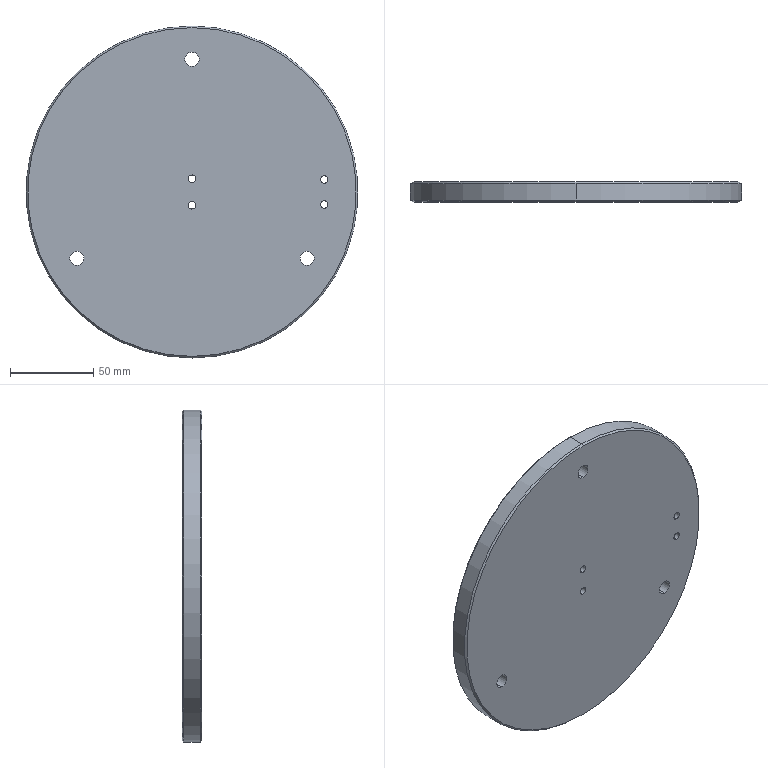Part | SolidWorks | features 3DProfileFeature 2, HoleWzd 2, Chamfer 1, Extrusion 1 | 1 solid | 34 faces | box 200 x 12 x 200 mm | volume 372597 mm3 | cylinder 24 | plane 6 | cone 4 | commonest cylinder face diameters 4.5 x8 8 x8 8.5 x6 200 x2
STEP:
#1=CARTESIAN_POINT('',(0.,-12.,-99.));
#2=VERTEX_POINT('',#1);
#3=CARTESIAN_POINT('',(0.,-12.,99.));
#4=VERTEX_POINT('',#3);
#5=CARTESIAN_POINT('',(0.,-12.,0.));
#6=DIRECTION('',(0.,-1.,0.));
#7=DIRECTION('',(0.,0.,1.));
#8=AXIS2_PLACEMENT_3D('',#5,#6,#7);
#9=CIRCLE('',#8,99.);
#10=EDGE_CURVE('',#2,#4,#9,.T.);
#11=ORIENTED_EDGE('',*,*,#10,.F.);
#12=CARTESIAN_POINT('',(0.,-11.,-100.));
#13=VERTEX_POINT('',#12);
#14=CARTESIAN_POINT('',(0.,-11.,-100.));
#15=DIRECTION('',(0.,0.7071,-0.7071));
#16=VECTOR('',#15,1000.);
#17=LINE('',#14,#16);
#18=EDGE_CURVE('',#2,#13,#17,.T.);
#19=ORIENTED_EDGE('',*,*,#18,.T.);
#20=CARTESIAN_POINT('',(0.,-11.,100.));
#21=VERTEX_POINT('',#20);
#22=CARTESIAN_POINT('',(0.,-11.,0.));
#23=DIRECTION('',(0.,1.,0.));
#24=DIRECTION('',(0.,0.,1.));
#25=AXIS2_PLACEMENT_3D('',#22,#23,#24);
#26=CIRCLE('',#25,100.);
#27=EDGE_CURVE('',#21,#13,#26,.T.);
#28=ORIENTED_EDGE('',*,*,#27,.F.);
#29=CARTESIAN_POINT('',(0.,-11.,100.));
#30=DIRECTION('',(0.,0.7071,0.7071));
#31=VECTOR('',#30,1000.);
#32=LINE('',#29,#31);
#33=EDGE_CURVE('',#4,#21,#32,.T.);
#34=ORIENTED_EDGE('',*,*,#33,.F.);
#35=EDGE_LOOP('',(#11,#19,#28,#34));
#36=FACE_OUTER_BOUND('',#35,.T.);
#37=CARTESIAN_POINT('',(0.,-11.,0.));
#38=DIRECTION('',(0.,1.,0.));
#39=DIRECTION('',(0.,0.,1.));
#40=AXIS2_PLACEMENT_3D('',#37,#38,#39);
#41=CONICAL_SURFACE('',#40,100.,0.7854);
#42=ADVANCED_FACE('',(#36),#41,.T.);
#43=CARTESIAN_POINT('',(0.,0.,99.));
#44=VERTEX_POINT('',#43);
#45=CARTESIAN_POINT('',(0.,0.,-99.));
#46=VERTEX_POINT('',#45);
#47=CARTESIAN_POINT('',(0.,0.,0.));
#48=DIRECTION('',(0.,1.,0.));
#49=DIRECTION('',(0.,0.,1.));
#50=AXIS2_PLACEMENT_3D('',#47,#48,#49);
#51=CIRCLE('',#50,99.);
#52=EDGE_CURVE('',#44,#46,#51,.T.);
#53=ORIENTED_EDGE('',*,*,#52,.F.);
#54=CARTESIAN_POINT('',(0.,-1.,100.));
#55=VERTEX_POINT('',#54);
#56=CARTESIAN_POINT('',(0.,0.,99.));
#57=DIRECTION('',(0.,-0.7071,0.7071));
#58=VECTOR('',#57,1000.);
#59=LINE('',#56,#58);
#60=EDGE_CURVE('',#44,#55,#59,.T.);
#61=ORIENTED_EDGE('',*,*,#60,.T.);
#62=CARTESIAN_POINT('',(0.,-1.,-100.));
#63=VERTEX_POINT('',#62);
#64=CARTESIAN_POINT('',(0.,-1.,0.));
#65=DIRECTION('',(0.,-1.,0.));
#66=DIRECTION('',(0.,0.,1.));
#67=AXIS2_PLACEMENT_3D('',#64,#65,#66);
#68=CIRCLE('',#67,100.);
#69=EDGE_CURVE('',#63,#55,#68,.T.);
#70=ORIENTED_EDGE('',*,*,#69,.F.);
#71=CARTESIAN_POINT('',(0.,0.,-99.));
#72=DIRECTION('',(0.,-0.7071,-0.7071));
#73=VECTOR('',#72,1000.);
#74=LINE('',#71,#73);
#75=EDGE_CURVE('',#46,#63,#74,.T.);
#76=ORIENTED_EDGE('',*,*,#75,.F.);
#77=EDGE_LOOP('',(#53,#61,#70,#76));
#78=FACE_OUTER_BOUND('',#77,.T.);
#79=CARTESIAN_POINT('',(0.,0.,0.));
#80=DIRECTION('',(0.,-1.,0.));
#81=DIRECTION('',(0.,0.,-1.));
#82=AXIS2_PLACEMENT_3D('',#79,#80,#81);
#83=CONICAL_SURFACE('',#82,99.,0.7854);
#84=ADVANCED_FACE('',(#78),#83,.T.);
#85=CARTESIAN_POINT('',(79.648,-7.,-11.5));
#86=VERTEX_POINT('',#85);
#87=CARTESIAN_POINT('',(79.648,-7.,-3.5));
#88=VERTEX_POINT('',#87);
#89=CARTESIAN_POINT('',(79.648,-7.,-7.5));
#90=DIRECTION('',(0.,1.,0.));
#91=DIRECTION('',(0.,0.,1.));
#92=AXIS2_PLACEMENT_3D('',#89,#90,#91);
#93=CIRCLE('',#92,4.);
#94=EDGE_CURVE('',#86,#88,#93,.T.);
#95=ORIENTED_EDGE('',*,*,#94,.F.);
#96=CARTESIAN_POINT('',(79.648,0.,-11.5));
#97=VERTEX_POINT('',#96);
#98=CARTESIAN_POINT('',(79.648,0.,-11.5));
#99=DIRECTION('',(0.,1.,0.));
#100=VECTOR('',#99,1000.);
#101=LINE('',#98,#100);
#102=EDGE_CURVE('',#86,#97,#101,.T.);
#103=ORIENTED_EDGE('',*,*,#102,.T.);
#104=CARTESIAN_POINT('',(79.648,0.,-3.5));
#105=VERTEX_POINT('',#104);
#106=CARTESIAN_POINT('',(79.648,0.,-7.5));
#107=DIRECTION('',(0.,1.,0.));
#108=DIRECTION('',(0.,0.,1.));
#109=AXIS2_PLACEMENT_3D('',#106,#107,#108);
#110=CIRCLE('',#109,4.);
#111=EDGE_CURVE('',#97,#105,#110,.T.);
#112=ORIENTED_EDGE('',*,*,#111,.T.);
#113=CARTESIAN_POINT('',(79.648,0.,-3.5));
#114=DIRECTION('',(0.,1.,0.));
#115=VECTOR('',#114,1000.);
#116=LINE('',#113,#115);
#117=EDGE_CURVE('',#88,#105,#116,.T.);
#118=ORIENTED_EDGE('',*,*,#117,.F.);
#119=EDGE_LOOP('',(#95,#103,#112,#118));
#120=FACE_OUTER_BOUND('',#119,.T.);
#121=CARTESIAN_POINT('',(79.648,0.,-7.5));
#122=DIRECTION('',(0.,1.,0.));
#123=DIRECTION('',(0.,0.,1.));
#124=AXIS2_PLACEMENT_3D('',#121,#122,#123);
#125=CYLINDRICAL_SURFACE('',#124,4.);
#126=ADVANCED_FACE('',(#120),#125,.F.);
#127=CARTESIAN_POINT('',(79.648,-12.,-9.75));
#128=VERTEX_POINT('',#127);
#129=CARTESIAN_POINT('',(79.648,-12.,-5.25));
#130=VERTEX_POINT('',#129);
#131=CARTESIAN_POINT('',(79.648,-12.,-7.5));
#132=DIRECTION('',(0.,1.,0.));
#133=DIRECTION('',(0.,0.,1.));
#134=AXIS2_PLACEMENT_3D('',#131,#132,#133);
#135=CIRCLE('',#134,2.25);
#136=EDGE_CURVE('',#128,#130,#135,.T.);
#137=ORIENTED_EDGE('',*,*,#136,.F.);
#138=CARTESIAN_POINT('',(79.648,-7.,-9.75));
#139=VERTEX_POINT('',#138);
#140=CARTESIAN_POINT('',(79.648,0.,-9.75));
#141=DIRECTION('',(0.,1.,0.));
#142=VECTOR('',#141,1000.);
#143=LINE('',#140,#142);
#144=EDGE_CURVE('',#128,#139,#143,.T.);
#145=ORIENTED_EDGE('',*,*,#144,.T.);
#146=CARTESIAN_POINT('',(79.648,-7.,-5.25));
#147=VERTEX_POINT('',#146);
#148=CARTESIAN_POINT('',(79.648,-7.,-7.5));
#149=DIRECTION('',(0.,1.,0.));
#150=DIRECTION('',(0.,0.,1.));
#151=AXIS2_PLACEMENT_3D('',#148,#149,#150);
#152=CIRCLE('',#151,2.25);
#153=EDGE_CURVE('',#139,#147,#152,.T.);
#154=ORIENTED_EDGE('',*,*,#153,.T.);
#155=CARTESIAN_POINT('',(79.648,0.,-5.25));
#156=DIRECTION('',(0.,1.,0.));
#157=VECTOR('',#156,1000.);
#158=LINE('',#155,#157);
#159=EDGE_CURVE('',#130,#147,#158,.T.);
#160=ORIENTED_EDGE('',*,*,#159,.F.);
#161=EDGE_LOOP('',(#137,#145,#154,#160));
#162=FACE_OUTER_BOUND('',#161,.T.);
#163=CARTESIAN_POINT('',(79.648,0.,-7.5));
#164=DIRECTION('',(0.,1.,0.));
#165=DIRECTION('',(0.,0.,1.));
#166=AXIS2_PLACEMENT_3D('',#163,#164,#165);
#167=CYLINDRICAL_SURFACE('',#166,2.25);
#168=ADVANCED_FACE('',(#162),#167,.F.);
#169=CARTESIAN_POINT('',(79.648,-7.,3.5));
#170=VERTEX_POINT('',#169);
#171=CARTESIAN_POINT('',(79.648,-7.,11.5));
#172=VERTEX_POINT('',#171);
#173=CARTESIAN_POINT('',(79.648,-7.,7.5));
#174=DIRECTION('',(0.,1.,0.));
#175=DIRECTION('',(0.,0.,1.));
#176=AXIS2_PLACEMENT_3D('',#173,#174,#175);
#177=CIRCLE('',#176,4.);
#178=EDGE_CURVE('',#170,#172,#177,.T.);
#179=ORIENTED_EDGE('',*,*,#178,.F.);
#180=CARTESIAN_POINT('',(79.648,0.,3.5));
#181=VERTEX_POINT('',#180);
#182=CARTESIAN_POINT('',(79.648,0.,3.5));
#183=DIRECTION('',(0.,1.,0.));
#184=VECTOR('',#183,1000.);
#185=LINE('',#182,#184);
#186=EDGE_CURVE('',#170,#181,#185,.T.);
#187=ORIENTED_EDGE('',*,*,#186,.T.);
#188=CARTESIAN_POINT('',(79.648,0.,11.5));
#189=VERTEX_POINT('',#188);
#190=CARTESIAN_POINT('',(79.648,0.,7.5));
#191=DIRECTION('',(0.,1.,0.));
#192=DIRECTION('',(0.,0.,1.));
#193=AXIS2_PLACEMENT_3D('',#190,#191,#192);
#194=CIRCLE('',#193,4.);
#195=EDGE_CURVE('',#181,#189,#194,.T.);
#196=ORIENTED_EDGE('',*,*,#195,.T.);
#197=CARTESIAN_POINT('',(79.648,0.,11.5));
#198=DIRECTION('',(0.,1.,0.));
#199=VECTOR('',#198,1000.);
#200=LINE('',#197,#199);
#201=EDGE_CURVE('',#172,#189,#200,.T.);
#202=ORIENTED_EDGE('',*,*,#201,.F.);
#203=EDGE_LOOP('',(#179,#187,#196,#202));
#204=FACE_OUTER_BOUND('',#203,.T.);
#205=CARTESIAN_POINT('',(79.648,0.,7.5));
#206=DIRECTION('',(0.,1.,0.));
#207=DIRECTION('',(0.,0.,1.));
#208=AXIS2_PLACEMENT_3D('',#205,#206,#207);
#209=CYLINDRICAL_SURFACE('',#208,4.);
#210=ADVANCED_FACE('',(#204),#209,.F.);
#211=CARTESIAN_POINT('',(79.648,-12.,5.25));
#212=VERTEX_POINT('',#211);
#213=CARTESIAN_POINT('',(79.648,-12.,9.75));
#214=VERTEX_POINT('',#213);
#215=CARTESIAN_POINT('',(79.648,-12.,7.5));
#216=DIRECTION('',(0.,1.,0.));
#217=DIRECTION('',(0.,0.,1.));
#218=AXIS2_PLACEMENT_3D('',#215,#216,#217);
#219=CIRCLE('',#218,2.25);
#220=EDGE_CURVE('',#212,#214,#219,.T.);
#221=ORIENTED_EDGE('',*,*,#220,.F.);
#222=CARTESIAN_POINT('',(79.648,-7.,5.25));
#223=VERTEX_POINT('',#222);
#224=CARTESIAN_POINT('',(79.648,0.,5.25));
#225=DIRECTION('',(0.,1.,0.));
#226=VECTOR('',#225,1000.);
#227=LINE('',#224,#226);
#228=EDGE_CURVE('',#212,#223,#227,.T.);
#229=ORIENTED_EDGE('',*,*,#228,.T.);
#230=CARTESIAN_POINT('',(79.648,-7.,9.75));
#231=VERTEX_POINT('',#230);
#232=CARTESIAN_POINT('',(79.648,-7.,7.5));
#233=DIRECTION('',(0.,1.,0.));
#234=DIRECTION('',(0.,0.,1.));
#235=AXIS2_PLACEMENT_3D('',#232,#233,#234);
#236=CIRCLE('',#235,2.25);
#237=EDGE_CURVE('',#223,#231,#236,.T.);
#238=ORIENTED_EDGE('',*,*,#237,.T.);
#239=CARTESIAN_POINT('',(79.648,0.,9.75));
#240=DIRECTION('',(0.,1.,0.));
#241=VECTOR('',#240,1000.);
#242=LINE('',#239,#241);
#243=EDGE_CURVE('',#214,#231,#242,.T.);
#244=ORIENTED_EDGE('',*,*,#243,.F.);
#245=EDGE_LOOP('',(#221,#229,#238,#244));
#246=FACE_OUTER_BOUND('',#245,.T.);
#247=CARTESIAN_POINT('',(79.648,0.,7.5));
#248=DIRECTION('',(0.,1.,0.));
#249=DIRECTION('',(0.,0.,1.));
#250=AXIS2_PLACEMENT_3D('',#247,#248,#249);
#251=CYLINDRICAL_SURFACE('',#250,2.25);
#252=ADVANCED_FACE('',(#246),#251,.F.);
#253=CARTESIAN_POINT('',(0.,-7.,4.));
#254=VERTEX_POINT('',#253);
#255=CARTESIAN_POINT('',(0.,-7.,12.));
#256=VERTEX_POINT('',#255);
#257=CARTESIAN_POINT('',(0.,-7.,8.));
#258=DIRECTION('',(0.,1.,0.));
#259=DIRECTION('',(0.,0.,1.));
#260=AXIS2_PLACEMENT_3D('',#257,#258,#259);
#261=CIRCLE('',#260,4.);
#262=EDGE_CURVE('',#254,#256,#261,.T.);
#263=ORIENTED_EDGE('',*,*,#262,.F.);
#264=CARTESIAN_POINT('',(0.,0.,4.));
#265=VERTEX_POINT('',#264);
#266=CARTESIAN_POINT('',(0.,0.,4.));
#267=DIRECTION('',(0.,1.,0.));
#268=VECTOR('',#267,1000.);
#269=LINE('',#266,#268);
#270=EDGE_CURVE('',#254,#265,#269,.T.);
#271=ORIENTED_EDGE('',*,*,#270,.T.);
#272=CARTESIAN_POINT('',(0.,0.,12.));
#273=VERTEX_POINT('',#272);
#274=CARTESIAN_POINT('',(0.,0.,8.));
#275=DIRECTION('',(0.,1.,0.));
#276=DIRECTION('',(0.,0.,1.));
#277=AXIS2_PLACEMENT_3D('',#274,#275,#276);
#278=CIRCLE('',#277,4.);
#279=EDGE_CURVE('',#265,#273,#278,.T.);
#280=ORIENTED_EDGE('',*,*,#279,.T.);
#281=CARTESIAN_POINT('',(0.,0.,12.));
#282=DIRECTION('',(0.,1.,0.));
#283=VECTOR('',#282,1000.);
#284=LINE('',#281,#283);
#285=EDGE_CURVE('',#256,#273,#284,.T.);
#286=ORIENTED_EDGE('',*,*,#285,.F.);
#287=EDGE_LOOP('',(#263,#271,#280,#286));
#288=FACE_OUTER_BOUND('',#287,.T.);
#289=CARTESIAN_POINT('',(0.,0.,8.));
#290=DIRECTION('',(0.,1.,0.));
#291=DIRECTION('',(0.,0.,1.));
#292=AXIS2_PLACEMENT_3D('',#289,#290,#291);
#293=CYLINDRICAL_SURFACE('',#292,4.);
#294=ADVANCED_FACE('',(#288),#293,.F.);
#295=CARTESIAN_POINT('',(0.,-12.,5.75));
#296=VERTEX_POINT('',#295);
#297=CARTESIAN_POINT('',(0.,-12.,10.25));
#298=VERTEX_POINT('',#297);
#299=CARTESIAN_POINT('',(0.,-12.,8.));
#300=DIRECTION('',(0.,1.,0.));
#301=DIRECTION('',(0.,0.,1.));
#302=AXIS2_PLACEMENT_3D('',#299,#300,#301);
#303=CIRCLE('',#302,2.25);
#304=EDGE_CURVE('',#296,#298,#303,.T.);
#305=ORIENTED_EDGE('',*,*,#304,.F.);
#306=CARTESIAN_POINT('',(0.,-7.,5.75));
#307=VERTEX_POINT('',#306);
#308=CARTESIAN_POINT('',(0.,0.,5.75));
#309=DIRECTION('',(0.,1.,0.));
#310=VECTOR('',#309,1000.);
#311=LINE('',#308,#310);
#312=EDGE_CURVE('',#296,#307,#311,.T.);
#313=ORIENTED_EDGE('',*,*,#312,.T.);
#314=CARTESIAN_POINT('',(0.,-7.,10.25));
#315=VERTEX_POINT('',#314);
#316=CARTESIAN_POINT('',(0.,-7.,8.));
#317=DIRECTION('',(0.,1.,0.));
#318=DIRECTION('',(0.,0.,1.));
#319=AXIS2_PLACEMENT_3D('',#316,#317,#318);
#320=CIRCLE('',#319,2.25);
#321=EDGE_CURVE('',#307,#315,#320,.T.);
#322=ORIENTED_EDGE('',*,*,#321,.T.);
#323=CARTESIAN_POINT('',(0.,0.,10.25));
#324=DIRECTION('',(0.,1.,0.));
#325=VECTOR('',#324,1000.);
#326=LINE('',#323,#325);
#327=EDGE_CURVE('',#298,#315,#326,.T.);
#328=ORIENTED_EDGE('',*,*,#327,.F.);
#329=EDGE_LOOP('',(#305,#313,#322,#328));
#330=FACE_OUTER_BOUND('',#329,.T.);
#331=CARTESIAN_POINT('',(0.,0.,8.));
#332=DIRECTION('',(0.,1.,0.));
#333=DIRECTION('',(0.,0.,1.));
#334=AXIS2_PLACEMENT_3D('',#331,#332,#333);
#335=CYLINDRICAL_SURFACE('',#334,2.25);
#336=ADVANCED_FACE('',(#330),#335,.F.);
#337=CARTESIAN_POINT('',(0.,-7.,-12.));
#338=VERTEX_POINT('',#337);
#339=CARTESIAN_POINT('',(0.,-7.,-4.));
#340=VERTEX_POINT('',#339);
#341=CARTESIAN_POINT('',(0.,-7.,-8.));
#342=DIRECTION('',(0.,1.,0.));
#343=DIRECTION('',(0.,0.,1.));
#344=AXIS2_PLACEMENT_3D('',#341,#342,#343);
#345=CIRCLE('',#344,4.);
#346=EDGE_CURVE('',#338,#340,#345,.T.);
#347=ORIENTED_EDGE('',*,*,#346,.F.);
#348=CARTESIAN_POINT('',(0.,0.,-12.));
#349=VERTEX_POINT('',#348);
#350=CARTESIAN_POINT('',(0.,0.,-12.));
#351=DIRECTION('',(0.,1.,0.));
#352=VECTOR('',#351,1000.);
#353=LINE('',#350,#352);
#354=EDGE_CURVE('',#338,#349,#353,.T.);
#355=ORIENTED_EDGE('',*,*,#354,.T.);
#356=CARTESIAN_POINT('',(0.,0.,-4.));
#357=VERTEX_POINT('',#356);
#358=CARTESIAN_POINT('',(0.,0.,-8.));
#359=DIRECTION('',(0.,1.,0.));
#360=DIRECTION('',(0.,0.,1.));
#361=AXIS2_PLACEMENT_3D('',#358,#359,#360);
#362=CIRCLE('',#361,4.);
#363=EDGE_CURVE('',#349,#357,#362,.T.);
#364=ORIENTED_EDGE('',*,*,#363,.T.);
#365=CARTESIAN_POINT('',(0.,0.,-4.));
#366=DIRECTION('',(0.,1.,0.));
#367=VECTOR('',#366,1000.);
#368=LINE('',#365,#367);
#369=EDGE_CURVE('',#340,#357,#368,.T.);
#370=ORIENTED_EDGE('',*,*,#369,.F.);
#371=EDGE_LOOP('',(#347,#355,#364,#370));
#372=FACE_OUTER_BOUND('',#371,.T.);
#373=CARTESIAN_POINT('',(0.,0.,-8.));
#374=DIRECTION('',(0.,1.,0.));
#375=DIRECTION('',(0.,0.,1.));
#376=AXIS2_PLACEMENT_3D('',#373,#374,#375);
#377=CYLINDRICAL_SURFACE('',#376,4.);
#378=ADVANCED_FACE('',(#372),#377,.F.);
#379=CARTESIAN_POINT('',(0.,-12.,-10.25));
#380=VERTEX_POINT('',#379);
#381=CARTESIAN_POINT('',(0.,-12.,-5.75));
#382=VERTEX_POINT('',#381);
#383=CARTESIAN_POINT('',(0.,-12.,-8.));
#384=DIRECTION('',(0.,1.,0.));
#385=DIRECTION('',(0.,0.,1.));
#386=AXIS2_PLACEMENT_3D('',#383,#384,#385);
#387=CIRCLE('',#386,2.25);
#388=EDGE_CURVE('',#380,#382,#387,.T.);
#389=ORIENTED_EDGE('',*,*,#388,.F.);
#390=CARTESIAN_POINT('',(0.,-7.,-10.25));
#391=VERTEX_POINT('',#390);
#392=CARTESIAN_POINT('',(0.,0.,-10.25));
#393=DIRECTION('',(0.,1.,0.));
#394=VECTOR('',#393,1000.);
#395=LINE('',#392,#394);
#396=EDGE_CURVE('',#380,#391,#395,.T.);
#397=ORIENTED_EDGE('',*,*,#396,.T.);
#398=CARTESIAN_POINT('',(0.,-7.,-5.75));
#399=VERTEX_POINT('',#398);
#400=CARTESIAN_POINT('',(0.,-7.,-8.));
#401=DIRECTION('',(0.,1.,0.));
#402=DIRECTION('',(0.,0.,1.));
#403=AXIS2_PLACEMENT_3D('',#400,#401,#402);
#404=CIRCLE('',#403,2.25);
#405=EDGE_CURVE('',#391,#399,#404,.T.);
#406=ORIENTED_EDGE('',*,*,#405,.T.);
#407=CARTESIAN_POINT('',(0.,0.,-5.75));
#408=DIRECTION('',(0.,1.,0.));
#409=VECTOR('',#408,1000.);
#410=LINE('',#407,#409);
#411=EDGE_CURVE('',#382,#399,#410,.T.);
#412=ORIENTED_EDGE('',*,*,#411,.F.);
#413=EDGE_LOOP('',(#389,#397,#406,#412));
#414=FACE_OUTER_BOUND('',#413,.T.);
#415=CARTESIAN_POINT('',(0.,0.,-8.));
#416=DIRECTION('',(0.,1.,0.));
#417=DIRECTION('',(0.,0.,1.));
#418=AXIS2_PLACEMENT_3D('',#415,#416,#417);
#419=CYLINDRICAL_SURFACE('',#418,2.25);
#420=ADVANCED_FACE('',(#414),#419,.F.);
#421=CARTESIAN_POINT('',(-69.282,-12.,-44.25));
#422=VERTEX_POINT('',#421);
#423=CARTESIAN_POINT('',(-69.282,-12.,-35.75));
#424=VERTEX_POINT('',#423);
#425=CARTESIAN_POINT('',(-69.282,-12.,-40.));
#426=DIRECTION('',(0.,1.,0.));
#427=DIRECTION('',(0.,0.,1.));
#428=AXIS2_PLACEMENT_3D('',#425,#426,#427);
#429=CIRCLE('',#428,4.25);
#430=EDGE_CURVE('',#422,#424,#429,.T.);
#431=ORIENTED_EDGE('',*,*,#430,.F.);
#432=CARTESIAN_POINT('',(-69.282,0.,-44.25));
#433=VERTEX_POINT('',#432);
#434=CARTESIAN_POINT('',(-69.282,0.,-44.25));
#435=DIRECTION('',(0.,1.,0.));
#436=VECTOR('',#435,1000.);
#437=LINE('',#434,#436);
#438=EDGE_CURVE('',#422,#433,#437,.T.);
#439=ORIENTED_EDGE('',*,*,#438,.T.);
#440=CARTESIAN_POINT('',(-69.282,0.,-35.75));
#441=VERTEX_POINT('',#440);
#442=CARTESIAN_POINT('',(-69.282,0.,-40.));
#443=DIRECTION('',(0.,1.,0.));
#444=DIRECTION('',(0.,0.,1.));
#445=AXIS2_PLACEMENT_3D('',#442,#443,#444);
#446=CIRCLE('',#445,4.25);
#447=EDGE_CURVE('',#433,#441,#446,.T.);
#448=ORIENTED_EDGE('',*,*,#447,.T.);
#449=CARTESIAN_POINT('',(-69.282,0.,-35.75));
#450=DIRECTION('',(0.,1.,0.));
#451=VECTOR('',#450,1000.);
#452=LINE('',#449,#451);
#453=EDGE_CURVE('',#424,#441,#452,.T.);
#454=ORIENTED_EDGE('',*,*,#453,.F.);
#455=EDGE_LOOP('',(#431,#439,#448,#454));
#456=FACE_OUTER_BOUND('',#455,.T.);
#457=CARTESIAN_POINT('',(-69.282,0.,-40.));
#458=DIRECTION('',(0.,1.,0.));
#459=DIRECTION('',(0.,0.,1.));
#460=AXIS2_PLACEMENT_3D('',#457,#458,#459);
#461=CYLINDRICAL_SURFACE('',#460,4.25);
#462=ADVANCED_FACE('',(#456),#461,.F.);
#463=CARTESIAN_POINT('',(69.282,-12.,-44.25));
#464=VERTEX_POINT('',#463);
#465=CARTESIAN_POINT('',(69.282,-12.,-35.75));
#466=VERTEX_POINT('',#465);
#467=CARTESIAN_POINT('',(69.282,-12.,-40.));
#468=DIRECTION('',(0.,1.,0.));
#469=DIRECTION('',(0.,0.,1.));
#470=AXIS2_PLACEMENT_3D('',#467,#468,#469);
#471=CIRCLE('',#470,4.25);
#472=EDGE_CURVE('',#464,#466,#471,.T.);
#473=ORIENTED_EDGE('',*,*,#472,.F.);
#474=CARTESIAN_POINT('',(69.282,0.,-44.25));
#475=VERTEX_POINT('',#474);
#476=CARTESIAN_POINT('',(69.282,0.,-44.25));
#477=DIRECTION('',(0.,1.,0.));
#478=VECTOR('',#477,1000.);
#479=LINE('',#476,#478);
#480=EDGE_CURVE('',#464,#475,#479,.T.);
#481=ORIENTED_EDGE('',*,*,#480,.T.);
#482=CARTESIAN_POINT('',(69.282,0.,-35.75));
#483=VERTEX_POINT('',#482);
#484=CARTESIAN_POINT('',(69.282,0.,-40.));
#485=DIRECTION('',(0.,1.,0.));
#486=DIRECTION('',(0.,0.,1.));
#487=AXIS2_PLACEMENT_3D('',#484,#485,#486);
#488=CIRCLE('',#487,4.25);
#489=EDGE_CURVE('',#475,#483,#488,.T.);
#490=ORIENTED_EDGE('',*,*,#489,.T.);
#491=CARTESIAN_POINT('',(69.282,0.,-35.75));
#492=DIRECTION('',(0.,1.,0.));
#493=VECTOR('',#492,1000.);
#494=LINE('',#491,#493);
#495=EDGE_CURVE('',#466,#483,#494,.T.);
#496=ORIENTED_EDGE('',*,*,#495,.F.);
#497=EDGE_LOOP('',(#473,#481,#490,#496));
#498=FACE_OUTER_BOUND('',#497,.T.);
#499=CARTESIAN_POINT('',(69.282,0.,-40.));
#500=DIRECTION('',(0.,1.,0.));
#501=DIRECTION('',(0.,0.,1.));
#502=AXIS2_PLACEMENT_3D('',#499,#500,#501);
#503=CYLINDRICAL_SURFACE('',#502,4.25);
#504=ADVANCED_FACE('',(#498),#503,.F.);
#505=CARTESIAN_POINT('',(0.,-12.,75.75));
#506=VERTEX_POINT('',#505);
#507=CARTESIAN_POINT('',(0.,-12.,84.25));
#508=VERTEX_POINT('',#507);
#509=CARTESIAN_POINT('',(0.,-12.,80.));
#510=DIRECTION('',(0.,1.,0.));
#511=DIRECTION('',(0.,0.,1.));
#512=AXIS2_PLACEMENT_3D('',#509,#510,#511);
#513=CIRCLE('',#512,4.25);
#514=EDGE_CURVE('',#506,#508,#513,.T.);
#515=ORIENTED_EDGE('',*,*,#514,.F.);
#516=CARTESIAN_POINT('',(0.,0.,75.75));
#517=VERTEX_POINT('',#516);
#518=CARTESIAN_POINT('',(0.,0.,75.75));
#519=DIRECTION('',(0.,1.,0.));
#520=VECTOR('',#519,1000.);
#521=LINE('',#518,#520);
#522=EDGE_CURVE('',#506,#517,#521,.T.);
#523=ORIENTED_EDGE('',*,*,#522,.T.);
#524=CARTESIAN_POINT('',(0.,0.,84.25));
#525=VERTEX_POINT('',#524);
#526=CARTESIAN_POINT('',(0.,0.,80.));
#527=DIRECTION('',(0.,1.,0.));
#528=DIRECTION('',(0.,0.,1.));
#529=AXIS2_PLACEMENT_3D('',#526,#527,#528);
#530=CIRCLE('',#529,4.25);
#531=EDGE_CURVE('',#517,#525,#530,.T.);
#532=ORIENTED_EDGE('',*,*,#531,.T.);
#533=CARTESIAN_POINT('',(0.,0.,84.25));
#534=DIRECTION('',(0.,1.,0.));
#535=VECTOR('',#534,1000.);
#536=LINE('',#533,#535);
#537=EDGE_CURVE('',#508,#525,#536,.T.);
#538=ORIENTED_EDGE('',*,*,#537,.F.);
#539=EDGE_LOOP('',(#515,#523,#532,#538));
#540=FACE_OUTER_BOUND('',#539,.T.);
#541=CARTESIAN_POINT('',(0.,0.,80.));
#542=DIRECTION('',(0.,1.,0.));
#543=DIRECTION('',(0.,0.,1.));
#544=AXIS2_PLACEMENT_3D('',#541,#542,#543);
#545=CYLINDRICAL_SURFACE('',#544,4.25);
#546=ADVANCED_FACE('',(#540),#545,.F.);
#547=ORIENTED_EDGE('',*,*,#27,.T.);
#548=CARTESIAN_POINT('',(0.,-12.,-100.));
#549=DIRECTION('',(0.,1.,0.));
#550=VECTOR('',#549,1000.);
#551=LINE('',#548,#550);
#552=EDGE_CURVE('',#13,#63,#551,.T.);
#553=ORIENTED_EDGE('',*,*,#552,.T.);
#554=ORIENTED_EDGE('',*,*,#69,.T.);
#555=CARTESIAN_POINT('',(0.,-12.,100.));
#556=DIRECTION('',(0.,1.,0.));
#557=VECTOR('',#556,1000.);
#558=LINE('',#555,#557);
#559=EDGE_CURVE('',#21,#55,#558,.T.);
#560=ORIENTED_EDGE('',*,*,#559,.F.);
#561=EDGE_LOOP('',(#547,#553,#554,#560));
#562=FACE_OUTER_BOUND('',#561,.T.);
#563=CARTESIAN_POINT('',(0.,-12.,0.));
#564=DIRECTION('',(0.,1.,0.));
#565=DIRECTION('',(0.,0.,1.));
#566=AXIS2_PLACEMENT_3D('',#563,#564,#565);
#567=CYLINDRICAL_SURFACE('',#566,100.);
#568=ADVANCED_FACE('',(#562),#567,.T.);
#569=ORIENTED_EDGE('',*,*,#552,.F.);
#570=CARTESIAN_POINT('',(0.,-11.,0.));
#571=DIRECTION('',(0.,1.,0.));
#572=DIRECTION('',(0.,0.,1.));
#573=AXIS2_PLACEMENT_3D('',#570,#571,#572);
#574=CIRCLE('',#573,100.);
#575=EDGE_CURVE('',#13,#21,#574,.T.);
#576=ORIENTED_EDGE('',*,*,#575,.T.);
#577=ORIENTED_EDGE('',*,*,#559,.T.);
#578=CARTESIAN_POINT('',(0.,-1.,0.));
#579=DIRECTION('',(0.,-1.,0.));
#580=DIRECTION('',(0.,0.,1.));
#581=AXIS2_PLACEMENT_3D('',#578,#579,#580);
#582=CIRCLE('',#581,100.);
#583=EDGE_CURVE('',#55,#63,#582,.T.);
#584=ORIENTED_EDGE('',*,*,#583,.T.);
#585=EDGE_LOOP('',(#569,#576,#577,#584));
#586=FACE_OUTER_BOUND('',#585,.T.);
#587=CARTESIAN_POINT('',(0.,-12.,0.));
#588=DIRECTION('',(0.,1.,0.));
#589=DIRECTION('',(0.,0.,1.));
#590=AXIS2_PLACEMENT_3D('',#587,#588,#589);
#591=CYLINDRICAL_SURFACE('',#590,100.);
#592=ADVANCED_FACE('',(#586),#591,.T.);
#593=CARTESIAN_POINT('',(0.,-12.,0.));
#594=DIRECTION('',(0.,-1.,0.));
#595=DIRECTION('',(0.,0.,1.));
#596=AXIS2_PLACEMENT_3D('',#593,#594,#595);
#597=CIRCLE('',#596,99.);
#598=EDGE_CURVE('',#4,#2,#597,.T.);
#599=ORIENTED_EDGE('',*,*,#598,.T.);
#600=ORIENTED_EDGE('',*,*,#10,.T.);
#601=EDGE_LOOP('',(#599,#600));
#602=FACE_OUTER_BOUND('',#601,.T.);
#603=CARTESIAN_POINT('',(79.648,-12.,-7.5));
#604=DIRECTION('',(0.,1.,0.));
#605=DIRECTION('',(0.,0.,1.));
#606=AXIS2_PLACEMENT_3D('',#603,#604,#605);
#607=CIRCLE('',#606,2.25);
#608=EDGE_CURVE('',#130,#128,#607,.T.);
#609=ORIENTED_EDGE('',*,*,#608,.T.);
#610=ORIENTED_EDGE('',*,*,#136,.T.);
#611=EDGE_LOOP('',(#609,#610));
#612=FACE_BOUND('',#611,.T.);
#613=CARTESIAN_POINT('',(79.648,-12.,7.5));
#614=DIRECTION('',(0.,1.,0.));
#615=DIRECTION('',(0.,0.,1.));
#616=AXIS2_PLACEMENT_3D('',#613,#614,#615);
#617=CIRCLE('',#616,2.25);
#618=EDGE_CURVE('',#214,#212,#617,.T.);
#619=ORIENTED_EDGE('',*,*,#618,.T.);
#620=ORIENTED_EDGE('',*,*,#220,.T.);
#621=EDGE_LOOP('',(#619,#620));
#622=FACE_BOUND('',#621,.T.);
#623=CARTESIAN_POINT('',(0.,-12.,8.));
#624=DIRECTION('',(0.,1.,0.));
#625=DIRECTION('',(0.,0.,1.));
#626=AXIS2_PLACEMENT_3D('',#623,#624,#625);
#627=CIRCLE('',#626,2.25);
#628=EDGE_CURVE('',#298,#296,#627,.T.);
#629=ORIENTED_EDGE('',*,*,#628,.T.);
#630=ORIENTED_EDGE('',*,*,#304,.T.);
#631=EDGE_LOOP('',(#629,#630));
#632=FACE_BOUND('',#631,.T.);
#633=CARTESIAN_POINT('',(0.,-12.,-8.));
#634=DIRECTION('',(0.,1.,0.));
#635=DIRECTION('',(0.,0.,1.));
#636=AXIS2_PLACEMENT_3D('',#633,#634,#635);
#637=CIRCLE('',#636,2.25);
#638=EDGE_CURVE('',#382,#380,#637,.T.);
#639=ORIENTED_EDGE('',*,*,#638,.T.);
#640=ORIENTED_EDGE('',*,*,#388,.T.);
#641=EDGE_LOOP('',(#639,#640));
#642=FACE_BOUND('',#641,.T.);
#643=CARTESIAN_POINT('',(-69.282,-12.,-40.));
#644=DIRECTION('',(0.,1.,0.));
#645=DIRECTION('',(0.,0.,1.));
#646=AXIS2_PLACEMENT_3D('',#643,#644,#645);
#647=CIRCLE('',#646,4.25);
#648=EDGE_CURVE('',#424,#422,#647,.T.);
#649=ORIENTED_EDGE('',*,*,#648,.T.);
#650=ORIENTED_EDGE('',*,*,#430,.T.);
#651=EDGE_LOOP('',(#649,#650));
#652=FACE_BOUND('',#651,.T.);
#653=CARTESIAN_POINT('',(69.282,-12.,-40.));
#654=DIRECTION('',(0.,1.,0.));
#655=DIRECTION('',(0.,0.,1.));
#656=AXIS2_PLACEMENT_3D('',#653,#654,#655);
#657=CIRCLE('',#656,4.25);
#658=EDGE_CURVE('',#466,#464,#657,.T.);
#659=ORIENTED_EDGE('',*,*,#658,.T.);
#660=ORIENTED_EDGE('',*,*,#472,.T.);
#661=EDGE_LOOP('',(#659,#660));
#662=FACE_BOUND('',#661,.T.);
#663=CARTESIAN_POINT('',(0.,-12.,80.));
#664=DIRECTION('',(0.,1.,0.));
#665=DIRECTION('',(0.,0.,1.));
#666=AXIS2_PLACEMENT_3D('',#663,#664,#665);
#667=CIRCLE('',#666,4.25);
#668=EDGE_CURVE('',#508,#506,#667,.T.);
#669=ORIENTED_EDGE('',*,*,#668,.T.);
#670=ORIENTED_EDGE('',*,*,#514,.T.);
#671=EDGE_LOOP('',(#669,#670));
#672=FACE_BOUND('',#671,.T.);
#673=CARTESIAN_POINT('',(0.,-12.,0.));
#674=DIRECTION('',(0.,1.,0.));
#675=DIRECTION('',(0.,0.,1.));
#676=AXIS2_PLACEMENT_3D('',#673,#674,#675);
#677=PLANE('',#676);
#678=ADVANCED_FACE('',(#602,#612,#622,#632,#642,#652,#662,#672),#677,.F.);
#679=CARTESIAN_POINT('',(0.,0.,0.));
#680=DIRECTION('',(0.,1.,0.));
#681=DIRECTION('',(0.,0.,1.));
#682=AXIS2_PLACEMENT_3D('',#679,#680,#681);
#683=CIRCLE('',#682,99.);
#684=EDGE_CURVE('',#46,#44,#683,.T.);
#685=ORIENTED_EDGE('',*,*,#684,.T.);
#686=ORIENTED_EDGE('',*,*,#52,.T.);
#687=EDGE_LOOP('',(#685,#686));
#688=FACE_OUTER_BOUND('',#687,.T.);
#689=CARTESIAN_POINT('',(79.648,0.,-7.5));
#690=DIRECTION('',(0.,1.,0.));
#691=DIRECTION('',(0.,0.,1.));
#692=AXIS2_PLACEMENT_3D('',#689,#690,#691);
#693=CIRCLE('',#692,4.);
#694=EDGE_CURVE('',#105,#97,#693,.T.);
#695=ORIENTED_EDGE('',*,*,#694,.F.);
#696=ORIENTED_EDGE('',*,*,#111,.F.);
#697=EDGE_LOOP('',(#695,#696));
#698=FACE_BOUND('',#697,.T.);
#699=CARTESIAN_POINT('',(79.648,0.,7.5));
#700=DIRECTION('',(0.,1.,0.));
#701=DIRECTION('',(0.,0.,1.));
#702=AXIS2_PLACEMENT_3D('',#699,#700,#701);
#703=CIRCLE('',#702,4.);
#704=EDGE_CURVE('',#189,#181,#703,.T.);
#705=ORIENTED_EDGE('',*,*,#704,.F.);
#706=ORIENTED_EDGE('',*,*,#195,.F.);
#707=EDGE_LOOP('',(#705,#706));
#708=FACE_BOUND('',#707,.T.);
#709=CARTESIAN_POINT('',(0.,0.,8.));
#710=DIRECTION('',(0.,1.,0.));
#711=DIRECTION('',(0.,0.,1.));
#712=AXIS2_PLACEMENT_3D('',#709,#710,#711);
#713=CIRCLE('',#712,4.);
#714=EDGE_CURVE('',#273,#265,#713,.T.);
#715=ORIENTED_EDGE('',*,*,#714,.F.);
#716=ORIENTED_EDGE('',*,*,#279,.F.);
#717=EDGE_LOOP('',(#715,#716));
#718=FACE_BOUND('',#717,.T.);
#719=CARTESIAN_POINT('',(0.,0.,-8.));
#720=DIRECTION('',(0.,1.,0.));
#721=DIRECTION('',(0.,0.,1.));
#722=AXIS2_PLACEMENT_3D('',#719,#720,#721);
#723=CIRCLE('',#722,4.);
#724=EDGE_CURVE('',#357,#349,#723,.T.);
#725=ORIENTED_EDGE('',*,*,#724,.F.);
#726=ORIENTED_EDGE('',*,*,#363,.F.);
#727=EDGE_LOOP('',(#725,#726));
#728=FACE_BOUND('',#727,.T.);
#729=CARTESIAN_POINT('',(-69.282,0.,-40.));
#730=DIRECTION('',(0.,1.,0.));
#731=DIRECTION('',(0.,0.,1.));
#732=AXIS2_PLACEMENT_3D('',#729,#730,#731);
#733=CIRCLE('',#732,4.25);
#734=EDGE_CURVE('',#441,#433,#733,.T.);
#735=ORIENTED_EDGE('',*,*,#734,.F.);
#736=ORIENTED_EDGE('',*,*,#447,.F.);
#737=EDGE_LOOP('',(#735,#736));
#738=FACE_BOUND('',#737,.T.);
#739=CARTESIAN_POINT('',(69.282,0.,-40.));
#740=DIRECTION('',(0.,1.,0.));
#741=DIRECTION('',(0.,0.,1.));
#742=AXIS2_PLACEMENT_3D('',#739,#740,#741);
#743=CIRCLE('',#742,4.25);
#744=EDGE_CURVE('',#483,#475,#743,.T.);
#745=ORIENTED_EDGE('',*,*,#744,.F.);
#746=ORIENTED_EDGE('',*,*,#489,.F.);
#747=EDGE_LOOP('',(#745,#746));
#748=FACE_BOUND('',#747,.T.);
#749=CARTESIAN_POINT('',(0.,0.,80.));
#750=DIRECTION('',(0.,1.,0.));
#751=DIRECTION('',(0.,0.,1.));
#752=AXIS2_PLACEMENT_3D('',#749,#750,#751);
#753=CIRCLE('',#752,4.25);
#754=EDGE_CURVE('',#525,#517,#753,.T.);
#755=ORIENTED_EDGE('',*,*,#754,.F.);
#756=ORIENTED_EDGE('',*,*,#531,.F.);
#757=EDGE_LOOP('',(#755,#756));
#758=FACE_BOUND('',#757,.T.);
#759=CARTESIAN_POINT('',(0.,0.,0.));
#760=DIRECTION('',(0.,1.,0.));
#761=DIRECTION('',(0.,0.,1.));
#762=AXIS2_PLACEMENT_3D('',#759,#760,#761);
#763=PLANE('',#762);
#764=ADVANCED_FACE('',(#688,#698,#708,#718,#728,#738,#748,#758),#763,.T.);
#765=ORIENTED_EDGE('',*,*,#522,.F.);
#766=ORIENTED_EDGE('',*,*,#668,.F.);
#767=ORIENTED_EDGE('',*,*,#537,.T.);
#768=ORIENTED_EDGE('',*,*,#754,.T.);
#769=EDGE_LOOP('',(#765,#766,#767,#768));
#770=FACE_OUTER_BOUND('',#769,.T.);
#771=CARTESIAN_POINT('',(0.,0.,80.));
#772=DIRECTION('',(0.,1.,0.));
#773=DIRECTION('',(0.,0.,1.));
#774=AXIS2_PLACEMENT_3D('',#771,#772,#773);
#775=CYLINDRICAL_SURFACE('',#774,4.25);
#776=ADVANCED_FACE('',(#770),#775,.F.);
#777=ORIENTED_EDGE('',*,*,#480,.F.);
#778=ORIENTED_EDGE('',*,*,#658,.F.);
#779=ORIENTED_EDGE('',*,*,#495,.T.);
#780=ORIENTED_EDGE('',*,*,#744,.T.);
#781=EDGE_LOOP('',(#777,#778,#779,#780));
#782=FACE_OUTER_BOUND('',#781,.T.);
#783=CARTESIAN_POINT('',(69.282,0.,-40.));
#784=DIRECTION('',(0.,1.,0.));
#785=DIRECTION('',(0.,0.,1.));
#786=AXIS2_PLACEMENT_3D('',#783,#784,#785);
#787=CYLINDRICAL_SURFACE('',#786,4.25);
#788=ADVANCED_FACE('',(#782),#787,.F.);
#789=ORIENTED_EDGE('',*,*,#438,.F.);
#790=ORIENTED_EDGE('',*,*,#648,.F.);
#791=ORIENTED_EDGE('',*,*,#453,.T.);
#792=ORIENTED_EDGE('',*,*,#734,.T.);
#793=EDGE_LOOP('',(#789,#790,#791,#792));
#794=FACE_OUTER_BOUND('',#793,.T.);
#795=CARTESIAN_POINT('',(-69.282,0.,-40.));
#796=DIRECTION('',(0.,1.,0.));
#797=DIRECTION('',(0.,0.,1.));
#798=AXIS2_PLACEMENT_3D('',#795,#796,#797);
#799=CYLINDRICAL_SURFACE('',#798,4.25);
#800=ADVANCED_FACE('',(#794),#799,.F.);
#801=ORIENTED_EDGE('',*,*,#396,.F.);
#802=ORIENTED_EDGE('',*,*,#638,.F.);
#803=ORIENTED_EDGE('',*,*,#411,.T.);
#804=CARTESIAN_POINT('',(0.,-7.,-8.));
#805=DIRECTION('',(0.,1.,0.));
#806=DIRECTION('',(0.,0.,1.));
#807=AXIS2_PLACEMENT_3D('',#804,#805,#806);
#808=CIRCLE('',#807,2.25);
#809=EDGE_CURVE('',#399,#391,#808,.T.);
#810=ORIENTED_EDGE('',*,*,#809,.T.);
#811=EDGE_LOOP('',(#801,#802,#803,#810));
#812=FACE_OUTER_BOUND('',#811,.T.);
#813=CARTESIAN_POINT('',(0.,0.,-8.));
#814=DIRECTION('',(0.,1.,0.));
#815=DIRECTION('',(0.,0.,1.));
#816=AXIS2_PLACEMENT_3D('',#813,#814,#815);
#817=CYLINDRICAL_SURFACE('',#816,2.25);
#818=ADVANCED_FACE('',(#812),#817,.F.);
#819=ORIENTED_EDGE('',*,*,#809,.F.);
#820=ORIENTED_EDGE('',*,*,#405,.F.);
#821=EDGE_LOOP('',(#819,#820));
#822=FACE_BOUND('',#821,.T.);
#823=CARTESIAN_POINT('',(0.,-7.,-8.));
#824=DIRECTION('',(0.,1.,0.));
#825=DIRECTION('',(0.,0.,1.));
#826=AXIS2_PLACEMENT_3D('',#823,#824,#825);
#827=CIRCLE('',#826,4.);
#828=EDGE_CURVE('',#340,#338,#827,.T.);
#829=ORIENTED_EDGE('',*,*,#828,.T.);
#830=ORIENTED_EDGE('',*,*,#346,.T.);
#831=EDGE_LOOP('',(#829,#830));
#832=FACE_OUTER_BOUND('',#831,.T.);
#833=CARTESIAN_POINT('',(2.25,-7.,-8.));
#834=DIRECTION('',(0.,-1.,0.));
#835=DIRECTION('',(0.,0.,-1.));
#836=AXIS2_PLACEMENT_3D('',#833,#834,#835);
#837=PLANE('',#836);
#838=ADVANCED_FACE('',(#822,#832),#837,.F.);
#839=ORIENTED_EDGE('',*,*,#354,.F.);
#840=ORIENTED_EDGE('',*,*,#828,.F.);
#841=ORIENTED_EDGE('',*,*,#369,.T.);
#842=ORIENTED_EDGE('',*,*,#724,.T.);
#843=EDGE_LOOP('',(#839,#840,#841,#842));
#844=FACE_OUTER_BOUND('',#843,.T.);
#845=CARTESIAN_POINT('',(0.,0.,-8.));
#846=DIRECTION('',(0.,1.,0.));
#847=DIRECTION('',(0.,0.,1.));
#848=AXIS2_PLACEMENT_3D('',#845,#846,#847);
#849=CYLINDRICAL_SURFACE('',#848,4.);
#850=ADVANCED_FACE('',(#844),#849,.F.);
#851=ORIENTED_EDGE('',*,*,#312,.F.);
#852=ORIENTED_EDGE('',*,*,#628,.F.);
#853=ORIENTED_EDGE('',*,*,#327,.T.);
#854=CARTESIAN_POINT('',(0.,-7.,8.));
#855=DIRECTION('',(0.,1.,0.));
#856=DIRECTION('',(0.,0.,1.));
#857=AXIS2_PLACEMENT_3D('',#854,#855,#856);
#858=CIRCLE('',#857,2.25);
#859=EDGE_CURVE('',#315,#307,#858,.T.);
#860=ORIENTED_EDGE('',*,*,#859,.T.);
#861=EDGE_LOOP('',(#851,#852,#853,#860));
#862=FACE_OUTER_BOUND('',#861,.T.);
#863=CARTESIAN_POINT('',(0.,0.,8.));
#864=DIRECTION('',(0.,1.,0.));
#865=DIRECTION('',(0.,0.,1.));
#866=AXIS2_PLACEMENT_3D('',#863,#864,#865);
#867=CYLINDRICAL_SURFACE('',#866,2.25);
#868=ADVANCED_FACE('',(#862),#867,.F.);
#869=ORIENTED_EDGE('',*,*,#859,.F.);
#870=ORIENTED_EDGE('',*,*,#321,.F.);
#871=EDGE_LOOP('',(#869,#870));
#872=FACE_BOUND('',#871,.T.);
#873=CARTESIAN_POINT('',(0.,-7.,8.));
#874=DIRECTION('',(0.,1.,0.));
#875=DIRECTION('',(0.,0.,1.));
#876=AXIS2_PLACEMENT_3D('',#873,#874,#875);
#877=CIRCLE('',#876,4.);
#878=EDGE_CURVE('',#256,#254,#877,.T.);
#879=ORIENTED_EDGE('',*,*,#878,.T.);
#880=ORIENTED_EDGE('',*,*,#262,.T.);
#881=EDGE_LOOP('',(#879,#880));
#882=FACE_OUTER_BOUND('',#881,.T.);
#883=CARTESIAN_POINT('',(2.25,-7.,8.));
#884=DIRECTION('',(0.,-1.,0.));
#885=DIRECTION('',(0.,0.,-1.));
#886=AXIS2_PLACEMENT_3D('',#883,#884,#885);
#887=PLANE('',#886);
#888=ADVANCED_FACE('',(#872,#882),#887,.F.);
#889=ORIENTED_EDGE('',*,*,#270,.F.);
#890=ORIENTED_EDGE('',*,*,#878,.F.);
#891=ORIENTED_EDGE('',*,*,#285,.T.);
#892=ORIENTED_EDGE('',*,*,#714,.T.);
#893=EDGE_LOOP('',(#889,#890,#891,#892));
#894=FACE_OUTER_BOUND('',#893,.T.);
#895=CARTESIAN_POINT('',(0.,0.,8.));
#896=DIRECTION('',(0.,1.,0.));
#897=DIRECTION('',(0.,0.,1.));
#898=AXIS2_PLACEMENT_3D('',#895,#896,#897);
#899=CYLINDRICAL_SURFACE('',#898,4.);
#900=ADVANCED_FACE('',(#894),#899,.F.);
#901=ORIENTED_EDGE('',*,*,#228,.F.);
#902=ORIENTED_EDGE('',*,*,#618,.F.);
#903=ORIENTED_EDGE('',*,*,#243,.T.);
#904=CARTESIAN_POINT('',(79.648,-7.,7.5));
#905=DIRECTION('',(0.,1.,0.));
#906=DIRECTION('',(0.,0.,1.));
#907=AXIS2_PLACEMENT_3D('',#904,#905,#906);
#908=CIRCLE('',#907,2.25);
#909=EDGE_CURVE('',#231,#223,#908,.T.);
#910=ORIENTED_EDGE('',*,*,#909,.T.);
#911=EDGE_LOOP('',(#901,#902,#903,#910));
#912=FACE_OUTER_BOUND('',#911,.T.);
#913=CARTESIAN_POINT('',(79.648,0.,7.5));
#914=DIRECTION('',(0.,1.,0.));
#915=DIRECTION('',(0.,0.,1.));
#916=AXIS2_PLACEMENT_3D('',#913,#914,#915);
#917=CYLINDRICAL_SURFACE('',#916,2.25);
#918=ADVANCED_FACE('',(#912),#917,.F.);
#919=ORIENTED_EDGE('',*,*,#909,.F.);
#920=ORIENTED_EDGE('',*,*,#237,.F.);
#921=EDGE_LOOP('',(#919,#920));
#922=FACE_BOUND('',#921,.T.);
#923=CARTESIAN_POINT('',(79.648,-7.,7.5));
#924=DIRECTION('',(0.,1.,0.));
#925=DIRECTION('',(0.,0.,1.));
#926=AXIS2_PLACEMENT_3D('',#923,#924,#925);
#927=CIRCLE('',#926,4.);
#928=EDGE_CURVE('',#172,#170,#927,.T.);
#929=ORIENTED_EDGE('',*,*,#928,.T.);
#930=ORIENTED_EDGE('',*,*,#178,.T.);
#931=EDGE_LOOP('',(#929,#930));
#932=FACE_OUTER_BOUND('',#931,.T.);
#933=CARTESIAN_POINT('',(81.898,-7.,7.5));
#934=DIRECTION('',(0.,-1.,0.));
#935=DIRECTION('',(0.,0.,-1.));
#936=AXIS2_PLACEMENT_3D('',#933,#934,#935);
#937=PLANE('',#936);
#938=ADVANCED_FACE('',(#922,#932),#937,.F.);
#939=ORIENTED_EDGE('',*,*,#186,.F.);
#940=ORIENTED_EDGE('',*,*,#928,.F.);
#941=ORIENTED_EDGE('',*,*,#201,.T.);
#942=ORIENTED_EDGE('',*,*,#704,.T.);
#943=EDGE_LOOP('',(#939,#940,#941,#942));
#944=FACE_OUTER_BOUND('',#943,.T.);
#945=CARTESIAN_POINT('',(79.648,0.,7.5));
#946=DIRECTION('',(0.,1.,0.));
#947=DIRECTION('',(0.,0.,1.));
#948=AXIS2_PLACEMENT_3D('',#945,#946,#947);
#949=CYLINDRICAL_SURFACE('',#948,4.);
#950=ADVANCED_FACE('',(#944),#949,.F.);
#951=ORIENTED_EDGE('',*,*,#144,.F.);
#952=ORIENTED_EDGE('',*,*,#608,.F.);
#953=ORIENTED_EDGE('',*,*,#159,.T.);
#954=CARTESIAN_POINT('',(79.648,-7.,-7.5));
#955=DIRECTION('',(0.,1.,0.));
#956=DIRECTION('',(0.,0.,1.));
#957=AXIS2_PLACEMENT_3D('',#954,#955,#956);
#958=CIRCLE('',#957,2.25);
#959=EDGE_CURVE('',#147,#139,#958,.T.);
#960=ORIENTED_EDGE('',*,*,#959,.T.);
#961=EDGE_LOOP('',(#951,#952,#953,#960));
#962=FACE_OUTER_BOUND('',#961,.T.);
#963=CARTESIAN_POINT('',(79.648,0.,-7.5));
#964=DIRECTION('',(0.,1.,0.));
#965=DIRECTION('',(0.,0.,1.));
#966=AXIS2_PLACEMENT_3D('',#963,#964,#965);
#967=CYLINDRICAL_SURFACE('',#966,2.25);
#968=ADVANCED_FACE('',(#962),#967,.F.);
#969=ORIENTED_EDGE('',*,*,#959,.F.);
#970=ORIENTED_EDGE('',*,*,#153,.F.);
#971=EDGE_LOOP('',(#969,#970));
#972=FACE_BOUND('',#971,.T.);
#973=CARTESIAN_POINT('',(79.648,-7.,-7.5));
#974=DIRECTION('',(0.,1.,0.));
#975=DIRECTION('',(0.,0.,1.));
#976=AXIS2_PLACEMENT_3D('',#973,#974,#975);
#977=CIRCLE('',#976,4.);
#978=EDGE_CURVE('',#88,#86,#977,.T.);
#979=ORIENTED_EDGE('',*,*,#978,.T.);
#980=ORIENTED_EDGE('',*,*,#94,.T.);
#981=EDGE_LOOP('',(#979,#980));
#982=FACE_OUTER_BOUND('',#981,.T.);
#983=CARTESIAN_POINT('',(81.898,-7.,-7.5));
#984=DIRECTION('',(0.,-1.,0.));
#985=DIRECTION('',(0.,0.,-1.));
#986=AXIS2_PLACEMENT_3D('',#983,#984,#985);
#987=PLANE('',#986);
#988=ADVANCED_FACE('',(#972,#982),#987,.F.);
#989=ORIENTED_EDGE('',*,*,#102,.F.);
#990=ORIENTED_EDGE('',*,*,#978,.F.);
#991=ORIENTED_EDGE('',*,*,#117,.T.);
#992=ORIENTED_EDGE('',*,*,#694,.T.);
#993=EDGE_LOOP('',(#989,#990,#991,#992));
#994=FACE_OUTER_BOUND('',#993,.T.);
#995=CARTESIAN_POINT('',(79.648,0.,-7.5));
#996=DIRECTION('',(0.,1.,0.));
#997=DIRECTION('',(0.,0.,1.));
#998=AXIS2_PLACEMENT_3D('',#995,#996,#997);
#999=CYLINDRICAL_SURFACE('',#998,4.);
#1000=ADVANCED_FACE('',(#994),#999,.F.);
#1001=ORIENTED_EDGE('',*,*,#60,.F.);
#1002=ORIENTED_EDGE('',*,*,#684,.F.);
#1003=ORIENTED_EDGE('',*,*,#75,.T.);
#1004=ORIENTED_EDGE('',*,*,#583,.F.);
#1005=EDGE_LOOP('',(#1001,#1002,#1003,#1004));
#1006=FACE_OUTER_BOUND('',#1005,.T.);
#1007=CARTESIAN_POINT('',(0.,0.,0.));
#1008=DIRECTION('',(0.,-1.,0.));
#1009=DIRECTION('',(0.,0.,-1.));
#1010=AXIS2_PLACEMENT_3D('',#1007,#1008,#1009);
#1011=CONICAL_SURFACE('',#1010,99.,0.7854);
#1012=ADVANCED_FACE('',(#1006),#1011,.T.);
#1013=ORIENTED_EDGE('',*,*,#18,.F.);
#1014=ORIENTED_EDGE('',*,*,#598,.F.);
#1015=ORIENTED_EDGE('',*,*,#33,.T.);
#1016=ORIENTED_EDGE('',*,*,#575,.F.);
#1017=EDGE_LOOP('',(#1013,#1014,#1015,#1016));
#1018=FACE_OUTER_BOUND('',#1017,.T.);
#1019=CARTESIAN_POINT('',(0.,-11.,0.));
#1020=DIRECTION('',(0.,1.,0.));
#1021=DIRECTION('',(0.,0.,1.));
#1022=AXIS2_PLACEMENT_3D('',#1019,#1020,#1021);
#1023=CONICAL_SURFACE('',#1022,100.,0.7854);
#1024=ADVANCED_FACE('',(#1018),#1023,.T.);
#1025=CLOSED_SHELL('',(#42,#84,#126,#168,#210,#252,#294,#336,#378,#420,#462,#504,#546,#568,#592,#678,#764,#776,#788,#800,#818,#838,#850,#868,#888,#900,#918,#938,#950,#968,#988,#1000,#1012,#1024));
#1026=MANIFOLD_SOLID_BREP('',#1025);
#1027=CARTESIAN_POINT('',(0.,0.,0.));
#1028=DIRECTION('',(0.,0.,1.));
#1029=DIRECTION('',(1.,0.,0.));
#1030=AXIS2_PLACEMENT_3D('',#1027,#1028,#1029);
#1031=(LENGTH_UNIT()NAMED_UNIT(*)SI_UNIT(.MILLI.,.METRE.));
#1032=UNCERTAINTY_MEASURE_WITH_UNIT(LENGTH_MEASURE(0.00001),#1031,'','');
#1033=(NAMED_UNIT(*)PLANE_ANGLE_UNIT()SI_UNIT($,.RADIAN.));
#1034=(NAMED_UNIT(*)SI_UNIT($,.STERADIAN.)SOLID_ANGLE_UNIT());
#1035=(GEOMETRIC_REPRESENTATION_CONTEXT(3)GLOBAL_UNCERTAINTY_ASSIGNED_CONTEXT((#1032))GLOBAL_UNIT_ASSIGNED_CONTEXT((#1031,#1033,#1034))REPRESENTATION_CONTEXT('',''));
#1036=ADVANCED_BREP_SHAPE_REPRESENTATION('',(#1026,#1030),#1035);